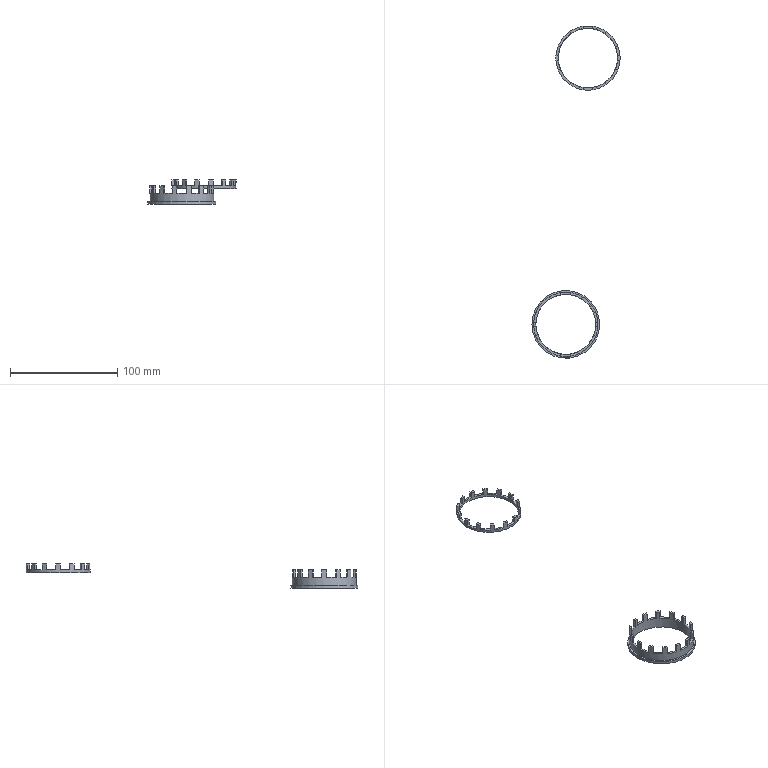NC program | NX | posted with a generic post | part box 82.344 x 310.506 x 22.5 mm
Lines 6896 to 7127 of 7127:
(PLANAR_MILL_1_COPY_13 , TOOL : D2A45)
N13712 T02 M6
N13714 G54
N13716 G17 G0 G90 X-21.916 Y-21.777 S9500 M3
N13718 G43 Z38. H2
N13720 Z3.
N13722 G94 G1 Z2. F1250.
N13724 G3 X-21.589 Y-21.403 R1.
N13726 G2 X-25.67 Y-16.285 R30.4
N13728 G3 X-26.107 Y-16.521 R1.
N13730 G1 Z3.
N13732 G0 Z38.
N13734 X-29.194 Y-10.111
N13736 Z3.
N13738 G1 Z2.
N13740 G3 X-28.737 Y-9.916 R1.
N13742 G2 X-30.194 Y-3.535 R30.4
N13744 G3 X-30.69 Y-3.557 R1.
N13746 G1 Z3.
N13748 G0 Z38.
N13750 Y3.557
N13752 Z3.
N13754 G1 Z2.
N13756 G3 X-30.194 Y3.535 R1.
N13758 G2 X-28.737 Y9.916 R30.4
N13760 G3 X-29.194 Y10.111 R1.
N13762 G1 Z3.
N13764 G0 Z38.
N13766 X-26.107 Y16.521
N13768 Z3.
N13770 G1 Z2.
N13772 G3 X-25.67 Y16.285 R1.
N13774 G2 X-21.589 Y21.403 R30.4
N13776 G3 X-21.916 Y21.777 R1.
N13778 G1 Z3.
N13780 G0 Z38.
N13782 X-16.354 Y26.212
N13784 Z3.
N13786 G1 Z2.
N13788 G3 X-16.062 Y25.81 R1.
N13790 G2 X-10.165 Y28.65 R30.4
N13792 G3 X-10.297 Y29.129 R1.
N13794 G1 Z3.
N13796 G0 Z38.
N13798 X-3.361 Y30.712
N13800 Z3.
N13802 G1 Z2.
N13804 G3 X-3.273 Y30.223 R1.
N13806 G2 X3.273 Y30.223 R30.4
N13808 G3 X3.361 Y30.712 R1.
N13810 G1 Z3.
N13812 G0 Z38.
N13814 X10.297 Y29.129
N13816 Z3.
N13818 G1 Z2.
N13820 G3 X10.165 Y28.65 R1.
N13822 G2 X16.062 Y25.81 R30.4
N13824 G3 X16.354 Y26.212 R1.
N13826 G1 Z3.
N13828 G0 Z38.
N13830 X21.916 Y21.777
N13832 Z3.
N13834 G1 Z2.
N13836 G3 X21.589 Y21.403 R1.
N13838 G2 X25.67 Y16.285 R30.4
N13840 G3 X26.107 Y16.521 R1.
N13842 G1 Z3.
N13844 G0 Z38.
N13846 X29.194 Y10.111
N13848 Z3.
N13850 G1 Z2.
N13852 G3 X28.737 Y9.916 R1.
N13854 G2 X30.194 Y3.535 R30.4
N13856 G3 X30.69 Y3.557 R1.
N13858 G1 Z3.
N13860 G0 Z38.
N13862 Y-3.557
N13864 Z3.
N13866 G1 Z2.
N13868 G3 X30.194 Y-3.535 R1.
N13870 G2 X28.737 Y-9.916 R30.4
N13872 G3 X29.194 Y-10.111 R1.
N13874 G1 Z3.
N13876 G0 Z38.
N13878 X26.107 Y-16.521
N13880 Z3.
N13882 G1 Z2.
N13884 G3 X25.67 Y-16.285 R1.
N13886 G2 X21.589 Y-21.403 R30.4
N13888 G3 X21.916 Y-21.777 R1.
N13890 G1 Z3.
N13892 G0 Z38.
N13894 X16.354 Y-26.212
N13896 Z3.
N13898 G1 Z2.
N13900 G3 X16.062 Y-25.81 R1.
N13902 G2 X10.165 Y-28.65 R30.4
N13904 G3 X10.297 Y-29.129 R1.
N13906 G1 Z3.
N13908 G0 Z38.
N13910 X3.361 Y-30.712
N13912 Z3.
N13914 G1 Z2.
N13916 G3 X3.273 Y-30.223 R1.
N13918 G2 X-3.273 Y-30.223 R30.4
N13920 G3 X-3.361 Y-30.712 R1.
N13922 G1 Z3.
N13924 G0 Z38.
N13926 X-10.297 Y-29.129
N13928 Z3.
N13930 G1 Z2.
N13932 G3 X-10.165 Y-28.65 R1.
N13934 G2 X-16.062 Y-25.81 R30.4
N13936 G3 X-16.354 Y-26.212 R1.
N13938 G1 Z3.
N13940 G0 Z38.
N13942 X-14.386 Y-22.675
N13944 Z3.
N13946 G1 Z2.
N13948 G3 X-14.641 Y-23.101 R1.
N13950 X-8.933 Y-25.85 R27.35
N13952 X-8.758 Y-25.385 R1.
N13954 G1 Z3.
N13956 G0 Z38.
N13958 X-3.123 Y-26.671
N13960 Z3.
N13962 G1 Z2.
N13964 G3 X-3.168 Y-27.166 R1.
N13966 X3.168 Y-27.166 R27.35
N13968 X3.123 Y-26.671 R1.
N13970 G1 Z3.
N13972 G0 Z38.
N13974 X8.758 Y-25.385
N13976 Z3.
N13978 G1 Z2.
N13980 G3 X8.933 Y-25.85 R1.
N13982 X14.641 Y-23.101 R27.35
N13984 X14.386 Y-22.675 R1.
N13986 G1 Z3.
N13988 G0 Z38.
N13990 X18.905 Y-19.071
N13992 Z3.
N13994 G1 Z2.
N13996 G3 X19.264 Y-19.414 R1.
N13998 X23.214 Y-14.461 R27.35
N14000 X22.799 Y-14.188 R1.
N14002 G1 Z3.
N14004 G0 Z38.
N14006 X25.308 Y-8.98
N14008 Z3.
N14010 G1 Z2.
N14012 G3 X25.78 Y-9.133 R1.
N14014 X27.19 Y-2.957 R27.35
N14016 X26.697 Y-2.89 R1.
N14018 G1 Z3.
N14020 G0 Z38.
N14022 Y2.89
N14024 Z3.
N14026 G1 Z2.
N14028 G3 X27.19 Y2.957 R1.
N14030 X25.78 Y9.133 R27.35
N14032 X25.308 Y8.98 R1.
N14034 G1 Z3.
N14036 G0 Z38.
N14038 X22.799 Y14.188
N14040 Z3.
N14042 G1 Z2.
N14044 G3 X23.214 Y14.461 R1.
N14046 X19.264 Y19.414 R27.35
N14048 X18.905 Y19.071 R1.
N14050 G1 Z3.
N14052 G0 Z38.
N14054 X14.386 Y22.675
N14056 Z3.
N14058 G1 Z2.
N14060 G3 X14.641 Y23.101 R1.
N14062 X8.933 Y25.85 R27.35
N14064 X8.758 Y25.385 R1.
N14066 G1 Z3.
N14068 G0 Z38.
N14070 X3.123 Y26.671
N14072 Z3.
N14074 G1 Z2.
N14076 G3 X3.168 Y27.166 R1.
N14078 X-3.168 Y27.166 R27.35
N14080 X-3.123 Y26.671 R1.
N14082 G1 Z3.
N14084 G0 Z38.
N14086 X-8.758 Y25.385
N14088 Z3.
N14090 G1 Z2.
N14092 G3 X-8.933 Y25.85 R1.
N14094 X-14.641 Y23.101 R27.35
N14096 X-14.386 Y22.675 R1.
N14098 G1 Z3.
N14100 G0 Z38.
N14102 X-18.905 Y19.071
N14104 Z3.
N14106 G1 Z2.
N14108 G3 X-19.264 Y19.414 R1.
N14110 X-23.214 Y14.461 R27.35
N14112 X-22.799 Y14.188 R1.
N14114 G1 Z3.
N14116 G0 Z38.
N14118 X-25.308 Y8.98
N14120 Z3.
N14122 G1 Z2.
N14124 G3 X-25.78 Y9.133 R1.
N14126 X-27.19 Y2.957 R27.35
N14128 X-26.697 Y2.89 R1.
N14130 G1 Z3.
N14132 G0 Z38.
N14134 Y-2.89
N14136 Z3.
N14138 G1 Z2.
N14140 G3 X-27.19 Y-2.957 R1.
N14142 X-25.78 Y-9.133 R27.35
N14144 X-25.308 Y-8.98 R1.
N14146 G1 Z3.
N14148 G0 Z38.
N14150 X-22.799 Y-14.188
N14152 Z3.
N14154 G1 Z2.
N14156 G3 X-23.214 Y-14.461 R1.
N14158 X-19.264 Y-19.414 R27.35
N14160 X-18.905 Y-19.071 R1.
N14162 G1 Z3.
N14164 G0 Z38.
N14166 M5
N14168 M2